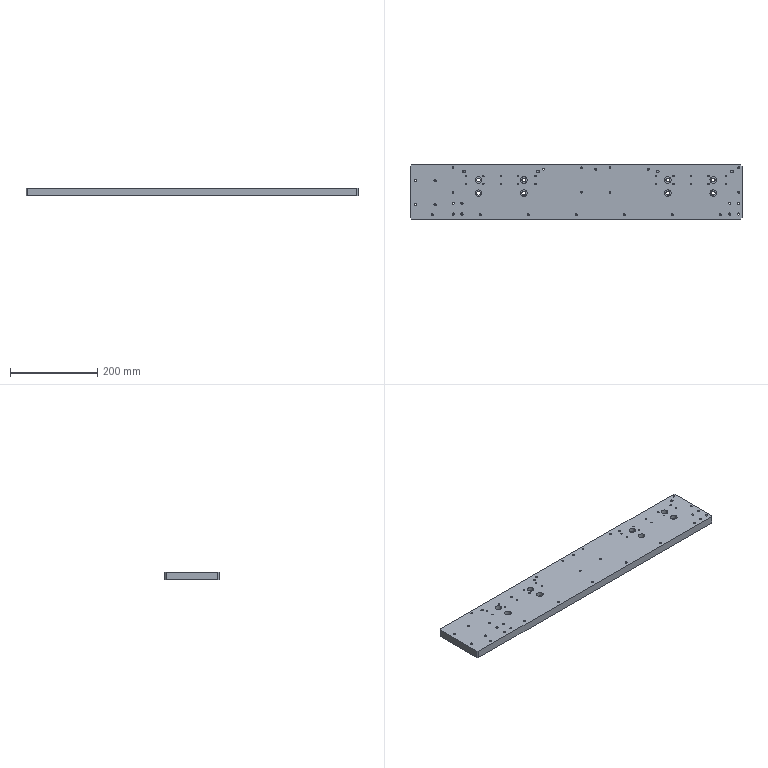Part | SolidWorks | features BaseBody 1 | 1 solid | 178 faces | box 761 x 125 x 18 mm | volume 1680532 mm3 | cylinder 146 | plane 18 | cone 14 | commonest cylinder face diameters 3.3 x46 5 x44 4.2 x16 9 x16 15 x16 6 x8